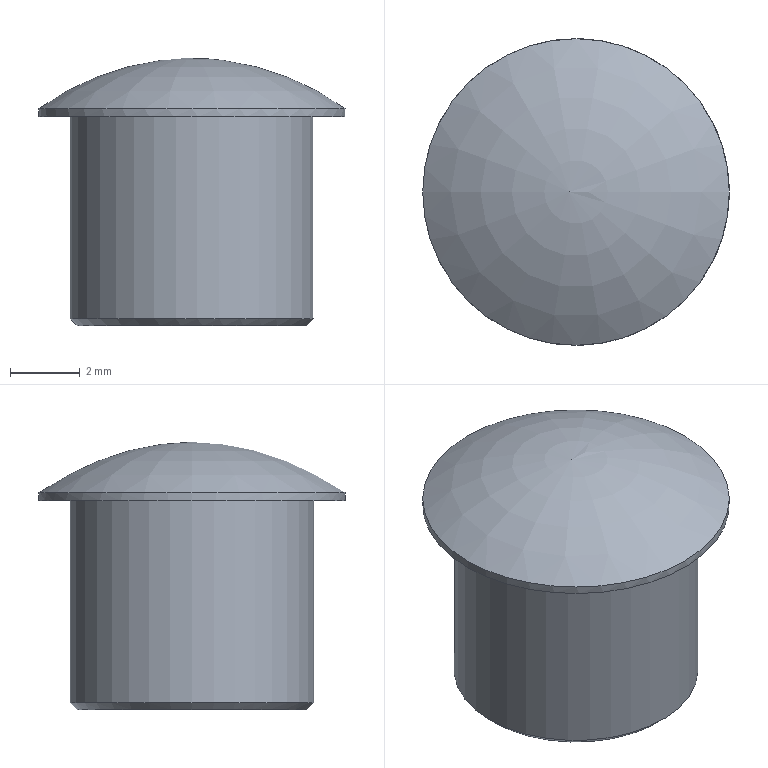Part | NX | features DATUM_CSYS 2, CHAMFER 1, SKETCH 1, SWP104 1 | 1 solid | 6 faces | box 8.8 x 8.8 x 7.684 mm | volume 289.37 mm3 | plane 2 | cylinder 2 | torus 1 | cone 1 | commonest cylinder face diameters 7 x1 8.8 x1
STEP:
#1=CARTESIAN_POINT('',(-3.3,0.,0.));
#2=VERTEX_POINT('',#1);
#3=CARTESIAN_POINT('',(0.,0.,0.));
#4=DIRECTION('',(0.,0.,-1.));
#5=DIRECTION('',(-1.,0.,0.));
#6=AXIS2_PLACEMENT_3D('',#3,#4,#5);
#7=CIRCLE('',#6,3.3);
#8=EDGE_CURVE('',#2,#2,#7,.T.);
#9=ORIENTED_EDGE('',*,*,#8,.T.);
#10=EDGE_LOOP('',(#9));
#11=FACE_BOUND('',#10,.T.);
#12=CARTESIAN_POINT('',(0.,0.,0.));
#13=DIRECTION('',(0.,0.,-1.));
#14=DIRECTION('',(-1.,0.,0.));
#15=AXIS2_PLACEMENT_3D('',#12,#13,#14);
#16=PLANE('',#15);
#17=ADVANCED_FACE('',(#11),#16,.T.);
#18=CARTESIAN_POINT('',(-3.5,0.,0.2));
#19=VERTEX_POINT('',#18);
#20=CARTESIAN_POINT('',(0.,0.,0.2));
#21=DIRECTION('',(0.,0.,-1.));
#22=DIRECTION('',(-1.,0.,0.));
#23=AXIS2_PLACEMENT_3D('',#20,#21,#22);
#24=CIRCLE('',#23,3.5);
#25=EDGE_CURVE('',#19,#19,#24,.F.);
#26=ORIENTED_EDGE('',*,*,#25,.T.);
#27=EDGE_LOOP('',(#26));
#28=FACE_BOUND('',#27,.T.);
#29=CARTESIAN_POINT('',(-3.5,0.,6.));
#30=VERTEX_POINT('',#29);
#31=CARTESIAN_POINT('',(0.,0.,6.));
#32=DIRECTION('',(0.,0.,-1.));
#33=DIRECTION('',(-1.,0.,0.));
#34=AXIS2_PLACEMENT_3D('',#31,#32,#33);
#35=CIRCLE('',#34,3.5);
#36=EDGE_CURVE('',#30,#30,#35,.T.);
#37=ORIENTED_EDGE('',*,*,#36,.T.);
#38=EDGE_LOOP('',(#37));
#39=FACE_BOUND('',#38,.T.);
#40=CARTESIAN_POINT('',(0.,0.,0.));
#41=DIRECTION('',(0.,0.,-1.));
#42=DIRECTION('',(-1.,0.,0.));
#43=AXIS2_PLACEMENT_3D('',#40,#41,#42);
#44=CYLINDRICAL_SURFACE('',#43,3.5);
#45=ADVANCED_FACE('',(#28,#39),#44,.T.);
#46=CARTESIAN_POINT('',(-4.4,0.,6.));
#47=VERTEX_POINT('',#46);
#48=CARTESIAN_POINT('',(0.,0.,6.));
#49=DIRECTION('',(0.,0.,-1.));
#50=DIRECTION('',(-1.,0.,0.));
#51=AXIS2_PLACEMENT_3D('',#48,#49,#50);
#52=CIRCLE('',#51,4.4);
#53=EDGE_CURVE('',#47,#47,#52,.T.);
#54=ORIENTED_EDGE('',*,*,#53,.T.);
#55=EDGE_LOOP('',(#54));
#56=FACE_BOUND('',#55,.T.);
#57=ORIENTED_EDGE('',*,*,#36,.F.);
#58=EDGE_LOOP('',(#57));
#59=FACE_BOUND('',#58,.T.);
#60=CARTESIAN_POINT('',(0.,3.5,6.));
#61=DIRECTION('',(0.,0.,-1.));
#62=DIRECTION('',(-1.,0.,0.));
#63=AXIS2_PLACEMENT_3D('',#60,#61,#62);
#64=PLANE('',#63);
#65=ADVANCED_FACE('',(#56,#59),#64,.T.);
#66=CARTESIAN_POINT('',(-4.4,0.,6.228));
#67=VERTEX_POINT('',#66);
#68=CARTESIAN_POINT('',(0.,0.,6.228));
#69=DIRECTION('',(0.,0.,-1.));
#70=DIRECTION('',(-1.,0.,0.));
#71=AXIS2_PLACEMENT_3D('',#68,#69,#70);
#72=CIRCLE('',#71,4.4);
#73=EDGE_CURVE('',#67,#67,#72,.T.);
#74=ORIENTED_EDGE('',*,*,#73,.T.);
#75=EDGE_LOOP('',(#74));
#76=FACE_BOUND('',#75,.T.);
#77=ORIENTED_EDGE('',*,*,#53,.F.);
#78=EDGE_LOOP('',(#77));
#79=FACE_BOUND('',#78,.T.);
#80=CARTESIAN_POINT('',(0.,0.,0.));
#81=DIRECTION('',(0.,0.,-1.));
#82=DIRECTION('',(-1.,0.,0.));
#83=AXIS2_PLACEMENT_3D('',#80,#81,#82);
#84=CYLINDRICAL_SURFACE('',#83,4.4);
#85=ADVANCED_FACE('',(#76,#79),#84,.T.);
#86=CARTESIAN_POINT('',(0.,0.,7.683));
#87=VERTEX_POINT('',#86);
#88=VERTEX_LOOP('',#87);
#89=FACE_BOUND('',#88,.T.);
#90=ORIENTED_EDGE('',*,*,#73,.F.);
#91=EDGE_LOOP('',(#90));
#92=FACE_BOUND('',#91,.T.);
#93=CARTESIAN_POINT('',(0.,0.,0.));
#94=DIRECTION('',(0.,0.,-1.));
#95=DIRECTION('',(-1.,0.,0.));
#96=AXIS2_PLACEMENT_3D('',#93,#94,#95);
#97=DEGENERATE_TOROIDAL_SURFACE('',#96,0.1,7.684,.F.);
#98=ADVANCED_FACE('',(#89,#92),#97,.F.);
#99=ORIENTED_EDGE('',*,*,#25,.F.);
#100=EDGE_LOOP('',(#99));
#101=FACE_BOUND('',#100,.T.);
#102=ORIENTED_EDGE('',*,*,#8,.F.);
#103=EDGE_LOOP('',(#102));
#104=FACE_BOUND('',#103,.T.);
#105=CARTESIAN_POINT('',(0.,0.,0.));
#106=DIRECTION('',(0.,0.,1.));
#107=DIRECTION('',(1.,0.,0.));
#108=AXIS2_PLACEMENT_3D('',#105,#106,#107);
#109=CONICAL_SURFACE('',#108,3.3,0.7854);
#110=ADVANCED_FACE('',(#101,#104),#109,.T.);
#111=CLOSED_SHELL('',(#17,#45,#65,#85,#98,#110));
#112=MANIFOLD_SOLID_BREP('',#111);
#113=(LENGTH_UNIT()NAMED_UNIT(*)SI_UNIT(.MILLI.,.METRE.));
#114=UNCERTAINTY_MEASURE_WITH_UNIT(LENGTH_MEASURE(0.00001),#113,'','');
#115=(NAMED_UNIT(*)PLANE_ANGLE_UNIT()SI_UNIT($,.RADIAN.));
#116=(NAMED_UNIT(*)SI_UNIT($,.STERADIAN.)SOLID_ANGLE_UNIT());
#117=(GEOMETRIC_REPRESENTATION_CONTEXT(3)GLOBAL_UNCERTAINTY_ASSIGNED_CONTEXT((#114))GLOBAL_UNIT_ASSIGNED_CONTEXT((#113,#115,#116))REPRESENTATION_CONTEXT('',''));
#118=ADVANCED_BREP_SHAPE_REPRESENTATION('',(#112),#117);